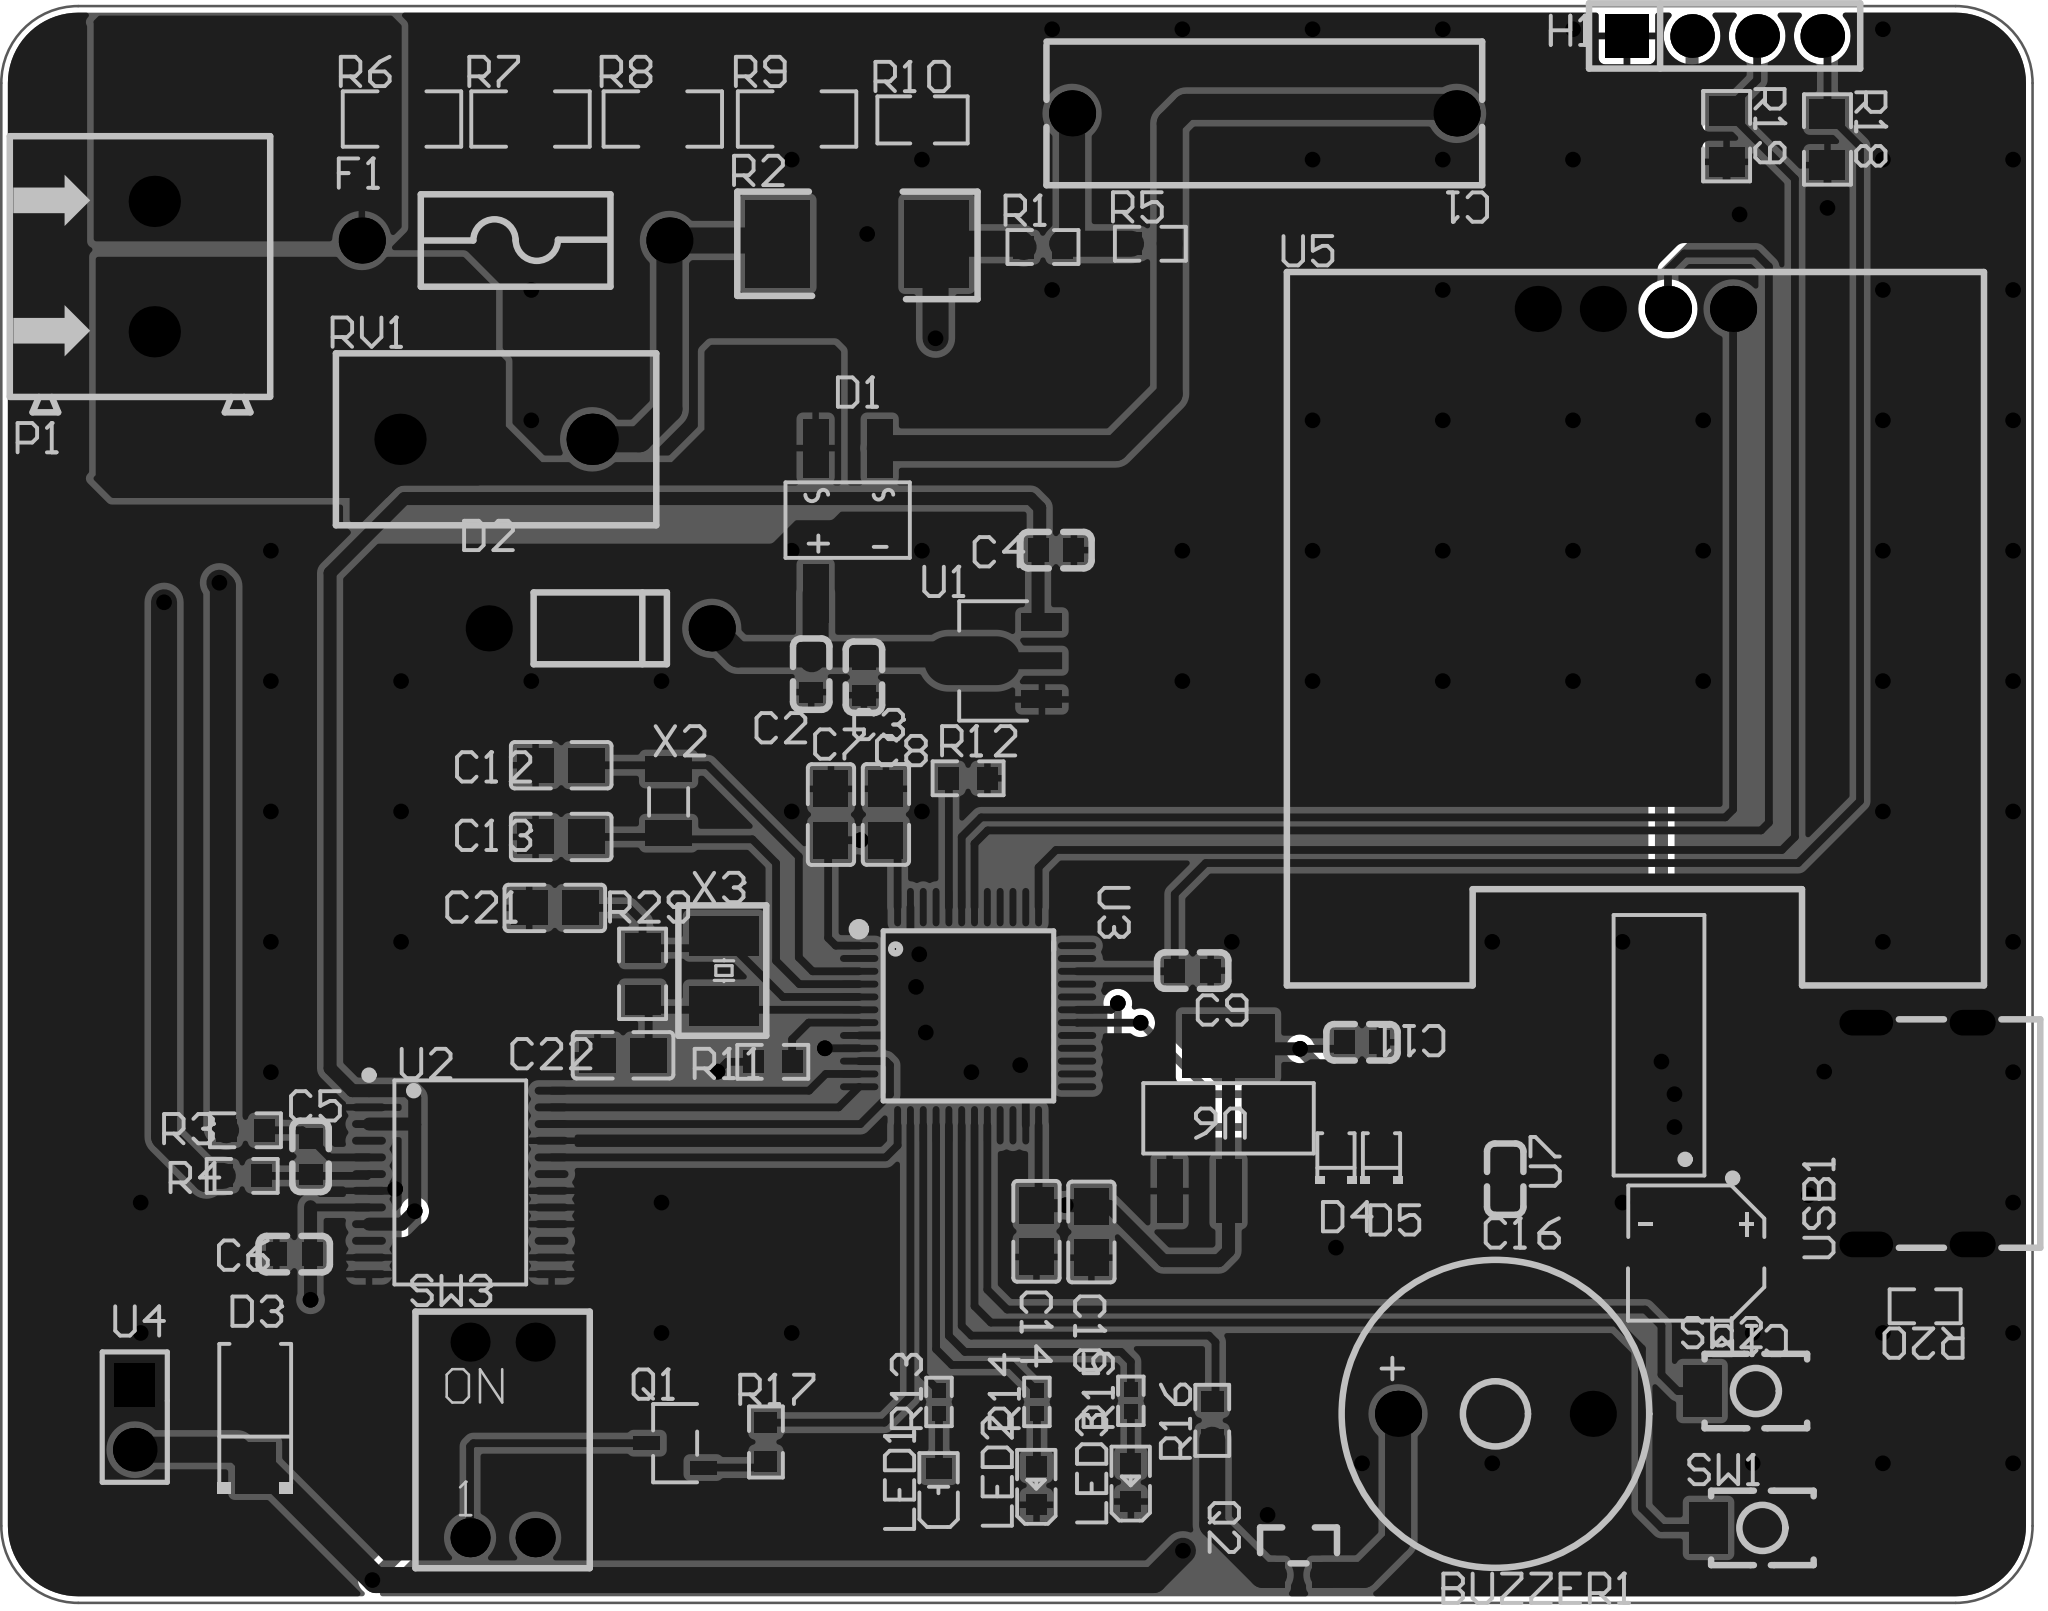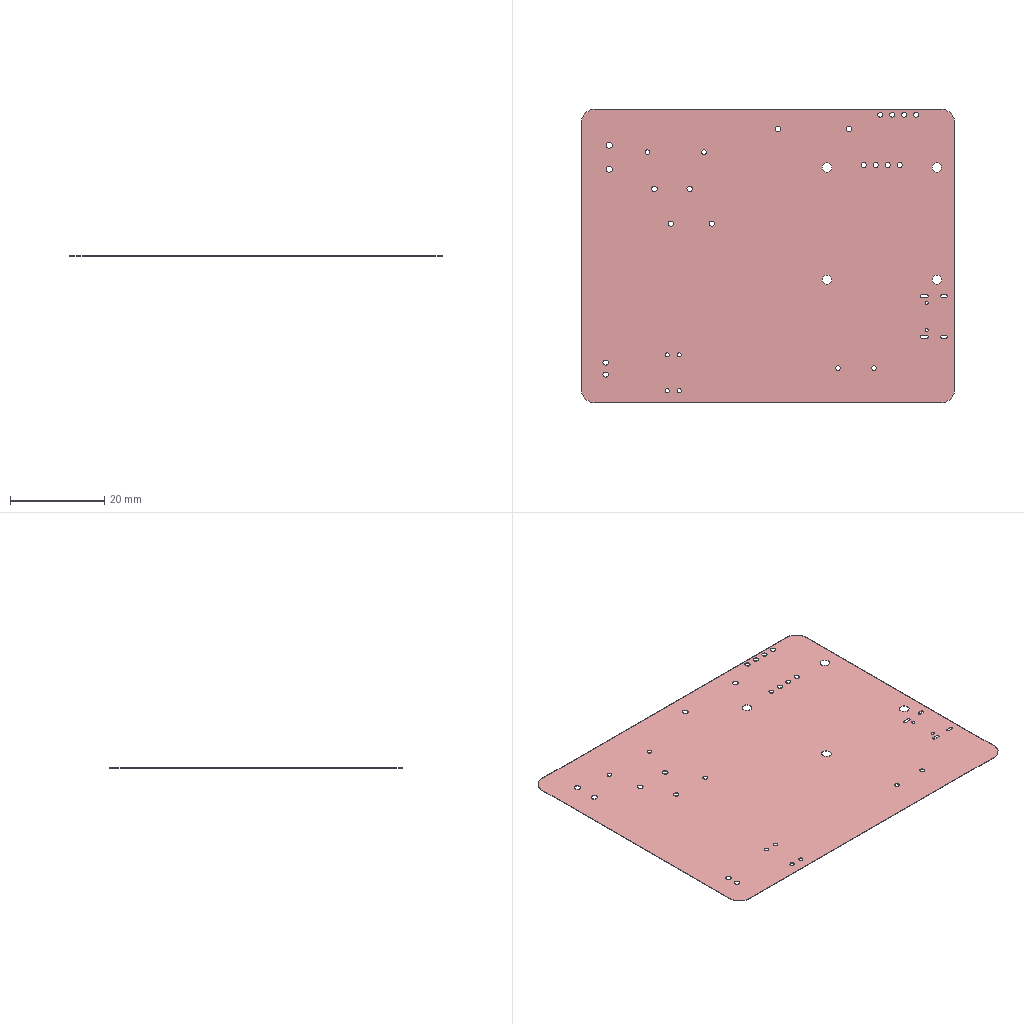Circuit board layout | Altium Designer | box 79.2 x 62.2 x 0.1 mm
Layer stack:
# Altium Designer layer stack of  (unit mm; dielectric type: 0 none, 1 core, 2 prepreg, 3 surface material)
index,name,kind,layer,copper_thickness_mm,dielectric_type,dielectric_thickness_mm,dielectric_material,dielectric_constant
0,Top Paste Mask Layer,other,,,,,,
1,Top Silkscreen Layer,other,,,,,,
2,Top Solder Mask Layer,dielectric,,,3,0.01,,3.3
3,Top Layer,copper,Top Layer,0.035,,,,
4,Bottom Layer,copper,Bottom Layer,0.035,,,,
5,Bottom Solder Mask Layer,dielectric,,,3,0.01,,3.3
6,Bottom Silkscreen Layer,other,,,,,,
7,Bottom Paste Mask Layer,other,,,,,,
# drill layer pairs: low layer,high layer
drill_pair,Top Layer,Bottom Layer
Part placement:
Designator,Comment,Layer,Footprint,Center-X(mm),Center-Y(mm),Rotation
BUZZER1,2.4kHz,TopLayer,BUZ-TH_BD12.0-P7.60-D0.6-FD,140.589,89.281,0
C1,470nF,TopLayer,CAP-TH_L17.0-W5.5-P15.00-D1.2,131.572,139.954,180
C3,0.1µF,TopLayer,C0603,115.951,117.983,270
C4,10µF,TopLayer,C0603,123.444,122.936,180
C5,1nF,TopLayer,C0603,94.361,99.314,90
C6,1nF,TopLayer,C0603,93.726,95.504,0
C7,100nF,TopLayer,C0805,114.665,112.633,90
C8,100nF,TopLayer,C0805,116.809,112.637,270
C14,100nF,TopLayer,C0805,122.682,96.393,90
C10,100nF,TopLayer,C0805,124.825,96.367,270
C11,100nF,TopLayer,C0603,135.382,103.759,180
D1,MB10S,TopLayer,MBS_L4.7-W4.0-P2.50-LS7.0-TL,115.316,124.079,270
D2,1N4742,TopLayer,DO-41_BD2.4-L4.7-P8.70-D0.8-FD,105.664,119.888,0
D3,1N4007,TopLayer,SMA_L4.3-W2.5-LS5.0-RD,92.202,89.281,90
F1,2F0.05002S1B02,TopLayer,FUSE-TH_BD3.0-L7.2-P11.20-D0.6,102.362,135.001,0
LED1,NCD0603G1,TopLayer,LED0603-RD_1,118.869,86.361,90
LED2,NCD0603R1,TopLayer,LED0603-RD_RED,122.682,86.487,90
LED3,NCD0603Y1,TopLayer,LED0603-RD,126.365,86.614,90
Q1,S8050 J3Y(RANGE:200-350),TopLayer,SOT-23-3_L3.0-W1.7-P0.95-LS2.9-BR,108.585,88.138,0
R1,10Ω,TopLayer,R0603,122.936,134.747,0
R2,2mΩ,TopLayer,RES-SMD_L6.4-W3.2-1,115.697,134.874,0
R3,1K,TopLayer,R0603,91.821,100.33,0
R4,1K,TopLayer,R0603,91.694,98.552,0
R5,1MΩ,TopLayer,R0603,127.127,134.874,0
R6,1MΩ,TopLayer,R1206,97.928,139.734,0
R7,1MΩ,TopLayer,R1206,102.943,139.734,0
R8,1MΩ,TopLayer,R1206,108.104,139.734,0
R9,1MΩ,TopLayer,R1206,113.342,139.734,0
R11,10K,TopLayer,R0603,112.395,102.997,0
R12,10K,TopLayer,R0603,120.015,114.046,0
R13,220Ω,TopLayer,R0402,118.879,89.745,90
R14,220Ω,TopLayer,R0402,122.7,89.745,90
R15,220Ω,TopLayer,R0402,126.365,89.789,90
R16,1KΩ,TopLayer,R0603,129.54,89.027,90
R17,1KΩ,TopLayer,R0603,112.128,88.184,270
RV1,190pF@1kHz,TopLayer,RES-TH_L12.5-W6.7-P7.50-D1.2,101.6,127.254,0
SW1,TS3425A2P 250gf,TopLayer,SW-SMD_L3.9-W2.9-LS5.0,151.003,84.836,0
SW2,TS3425A2P 250gf,TopLayer,SW-SMD_L3.9-W2.9-LS5.0,150.749,90.17,0
SW3,BSE02GR,TopLayer,SW-TH_4P-L9.9-W6.8-P7.62-BL,101.854,88.265,0
U1,HT7550-1,TopLayer,SOT-89_L4.5-W2.5-P1.50-LS4.2-BR,121.734,118.618,0
U2,ADE7755ARSZ,TopLayer,SSOP-24_L8.1-W5.3-P0.65-LS7.8-BL,100.203,98.298,270
U3,STM32F030C8T6TR,TopLayer,LQFP-48_L7.0-W7.0-P0.50-LS9.0-BL,120.015,104.775,270
U5,HS96L03W2C03,TopLayer,OLED-TH_L27.8-W27.2-P2.54_C9900033791,146.05,132.334,0
U6,AMS1117-3.3,TopLayer,SOT-223-4_L6.5-W3.5-P2.30-LS7.0-BR,130.175,100.796,270
P1,WJ500V-5.08-2P,TopLayer,CONN-TH_2P-P5.00_WJ500V-5.08-2P,88.265,133.985,90
U4,KF301-5.0-2P,TopLayer,HDR-M-2.54_1X2,87.503,89.154,270
C12,20pF,TopLayer,C0805,104.14,114.554,180
C13,20pF,TopLayer,C0805,104.14,111.76,0
C21,20pF,TopLayer,C0805,103.891,108.994,0
C22,20pF,TopLayer,C0805,106.553,103.251,0
R29,1M,TopLayer,R0805,107.315,106.426,90
X3,8MHz,TopLayer,CRYSTAL-SMD_L3.2-W2.5_3225-8MHZ,110.49,106.553,90
C9,100nF,TopLayer,C0603,128.778,106.553,180
C16,100nF,TopLayer,C0603,140.97,98.425,90
R18,10kΩ,TopLayer,R0805,153.543,138.938,270
R19,10kΩ,TopLayer,R0805,149.606,139.065,270
R20,5.1K,TopLayer,R0603,157.353,93.472,180
U7,CH340C,TopLayer,SOP-16_L10.0-W3.9-P1.27-LS6.0-BL,146.97,103.642,90
USB1,TYPE-C16PIN,TopLayer,USB-C-SMD_TYPE-C16PIN,156.845,100.203,90
Q2,,TopLayer,S8050_SOT-23,132.906,84.154,270
H1,,TopLayer,HDR-TH_4P-P2.54-V-F,149.53,142.971,0
D4,1N5819WS,TopLayer,SOD-323_L1.8-W1.3-LS2.5-RD,134.366,99.314,90
D5,1N5819WS,TopLayer,SOD-323_L1.8-W1.3-LS2.5-RD,136.144,99.314,90
C2,47uF,TopLayer,C0603,113.894,118.104,270
C15,10uF,TopLayer,CAP-SMD_BD5.0-L5.3-W5.3-FD,148.42,95.561,180
R10,10kΩ,TopLayer,R0805,118.237,139.7,0
X2,32.768kHz,TopLayer,CRYSTAL-SMD_L3.2-W1.5-FC-135R32.768KF-A3,108.331,113.157,270
Pad and via stacks:
# Altium Designer via and pad stacks of  (unit mm). Each distinct definition once, with the count of objects using it.
# via: kind,start_layer,end_layer,hole_mm,diameter_mm,mode(0 simple;1 top-mid-bottom;2 full stack),diameter_per_layer,count,example_net
# pad: kind,layer,hole_mm,hole_type(0 round;1 square;2 slot),plating,top_size,top_shape(1 round;2 rect;3 octagon;9 rounded rect),mid_size,bottom_size,mode,footprint,size_per_layer,count,example
pad,Multi-Layer,1,0,plated,1.8x1.8,1,1.8x1.8,1.8x1.8,0,BUZ-TH_BD12.0-P7.60-D0.6-FD,,2,BUZZER1.2
pad,Multi-Layer,1.2,0,plated,1.8x1.8,1,1.8x1.8,1.8x1.8,0,CAP-TH_L17.0-W5.5-P15.00-D1.2,,2,C1.1
pad,Multi-Layer,1.1,0,plated,1.8x1.8,1,1.8x1.8,1.8x1.8,0,DO-41_BD2.4-L4.7-P8.70-D0.8-FD,,2,D2.1
pad,Multi-Layer,1,0,plated,1.8x1.8,1,1.8x1.8,1.8x1.8,0,FUSE-TH_BD3.0-L7.2-P11.20-D0.6,,2,F1.1
pad,Multi-Layer,1.2,0,plated,2x2,1,2x2,2x2,0,RES-TH_L12.5-W6.7-P7.50-D1.2,,2,RV1.1
pad,Multi-Layer,0.9144,0,plated,1.524x1.524,1,1.524x1.524,1.524x1.524,0,SW-TH_4P-L9.9-W6.8-P7.62-BL,,4,SW3.1
pad,Multi-Layer,1.05,0,plated,1.8x1.8,1,1.8x1.8,1.8x1.8,0,OLED-TH_L27.8-W27.2-P2.54_C9900033791,,4,U5.1
pad,Multi-Layer,1.3,0,plated,2x2,1,2x2,2x2,0,CONN-TH_2P-P5.00_WJ500V-5.08-2P,,2,P1.2
pad,Multi-Layer,1.1,0,plated,1.7x1.575,2,1.7x1.575,1.7x1.575,0,HDR-M-2.54_1X2,,1,U4.1
pad,Multi-Layer,1.1,0,plated,1.7x1.7,1,1.7x1.7,1.7x1.7,0,HDR-M-2.54_1X2,,1,U4.2
pad,Multi-Layer,0.6,2,plated,1x1.8,1,1x1.8,1x1.8,0,USB-C-SMD_TYPE-C16PIN,,2,USB1.4
pad,Multi-Layer,0.6,2,plated,1x2.1,1,1x2.1,1x2.1,0,USB-C-SMD_TYPE-C16PIN,,2,USB1.2
pad,Multi-Layer,1.1,0,plated,1.7x1.7,2,1.7x1.7,1.7x1.7,0,HDR-TH_4P-P2.54-V-F,,1,H1.1
pad,Multi-Layer,1.1,0,plated,1.7x1.7,1,1.7x1.7,1.7x1.7,0,HDR-TH_4P-P2.54-V-F,,3,H1.2
pad,Top Layer,0,0,plated,0.8x0.9,2,0.8x0.9,0.8x0.9,0,C0603,,16,C3.2
pad,Top Layer,0,0,plated,1.41x1.35,2,1.41x1.35,1.41x1.35,0,C0805,,16,C7.2
pad,Top Layer,0,0,plated,0.98x2.265,2,0.98x2.265,0.98x2.265,0,MBS_L4.7-W4.0-P2.50-LS7.0-TL,,4,D1.1
pad,Top Layer,0,0,plated,2x1.593,2,2x1.593,2x1.593,0,SMA_L4.3-W2.5-LS5.0-RD,,2,D3.2
pad,Top Layer,0,0,plated,1x0.8,2,1x0.8,1x0.8,0,LED0603-RD_1,,2,LED1.2
pad,Top Layer,0,0,plated,0.8x0.8,2,0.8x0.8,0.8x0.8,0,LED0603-RD_RED,,2,LED2.1
pad,Top Layer,0,0,plated,0.8x0.8,2,0.8x0.8,0.8x0.8,0,LED0603-RD,,2,LED3.2
pad,Top Layer,0,0,plated,1.038x0.532,2,1.038x0.532,1.038x0.532,0,SOT-23-3_L3.0-W1.7-P0.95-LS2.9-BR,,3,Q1.1
pad,Top Layer,0,0,plated,0.8065x0.864,2,0.8065x0.864,0.8065x0.864,0,R0603,,18,R1.2
pad,Top Layer,0,0,plated,2.5x3.4,2,2.5x3.4,2.5x3.4,0,RES-SMD_L6.4-W3.2-1,,2,R2.2
pad,Top Layer,0,0,plated,1.208x1.701,2,1.208x1.701,1.208x1.701,0,R1206,,8,R6.2
pad,Top Layer,0,0,plated,0.5657x0.54,2,0.5657x0.54,0.5657x0.54,0,R0402,,6,R13.2
pad,Top Layer,0,0,plated,1.5x2,2,1.5x2,1.5x2,0,SW-SMD_L3.9-W2.9-LS5.0,,4,SW1.1
pad,Top Layer,0,0,plated,0.95x0.95,1,0.95x0.95,0.95x0.95,0,SOT-89_L4.5-W2.5-P1.50-LS4.2-BR,,1,U1.2
pad,Top Layer,0,0,plated,1.575x0.672,2,1.575x0.672,1.575x0.672,0,SOT-89_L4.5-W2.5-P1.50-LS4.2-BR,,2,U1.3
pad,Top Layer,0,0,plated,0.308x1.324,1,0.308x1.324,0.308x1.324,0,SSOP-24_L8.1-W5.3-P0.65-LS7.8-BL,,24,U2.1
pad,Top Layer,0,0,plated,0.27x1.5,1,0.27x1.5,0.27x1.5,0,LQFP-48_L7.0-W7.0-P0.50-LS9.0-BL,,24,U3.1
pad,Top Layer,0,0,plated,1.5x0.27,1,1.5x0.27,1.5x0.27,0,LQFP-48_L7.0-W7.0-P0.50-LS9.0-BL,,24,U3.13
pad,Top Layer,0,0,plated,2.47x0.98,2,2.47x0.98,2.47x0.98,0,SOT-223-4_L6.5-W3.5-P2.30-LS7.0-BR,,3,U6.1
pad,Top Layer,0,0,plated,2.47x3.6,2,2.47x3.6,2.47x3.6,0,SOT-223-4_L6.5-W3.5-P2.30-LS7.0-BR,,1,U6.4
pad,Top Layer,0,0,plated,1.133x1.377,2,1.133x1.377,1.133x1.377,0,R0805,,8,R29.2
pad,Top Layer,0,0,plated,1.524x2.7,2,1.524x2.7,1.524x2.7,0,CRYSTAL-SMD_L3.2-W2.5_3225-8MHZ,,2,X3.1
pad,Top Layer,0,0,plated,0.56x1.745,1,0.56x1.745,0.56x1.745,0,SOP-16_L10.0-W3.9-P1.27-LS6.0-BL,,16,U7.1
pad,Top Layer,0,0,plated,0.6x1.15,2,0.6x1.15,0.6x1.15,0,USB-C-SMD_TYPE-C16PIN,,4,USB1.A1B12
pad,Top Layer,0,0,plated,0.3x1.15,2,0.3x1.15,0.3x1.15,0,USB-C-SMD_TYPE-C16PIN,,8,USB1.B5
pad,Top Layer,0,0,plated,1x0.8,2,1x0.8,1x0.8,0,S8050_SOT-23,,3,Q2.2
pad,Top Layer,0,0,plated,1x0.75,2,1x0.75,1x0.75,0,SOD-323_L1.8-W1.3-LS2.5-RD,,4,D4.1
pad,Top Layer,0,0,plated,2.8x1.1,2,2.8x1.1,2.8x1.1,0,CAP-SMD_BD5.0-L5.3-W5.3-FD,,2,C15.1
pad,Top Layer,0,0,plated,1x1.8,2,1x1.8,1x1.8,0,CRYSTAL-SMD_L3.2-W1.5-FC-135R32.768KF-A3,,2,X2.2
via,Top Layer,Bottom Layer,0.3048,0.6096,0,,106,TT1
Copper pours:
name,layer,net,type(0 solid;1 hatched;2 none)
Top Layer-$1N1,Top Layer,$1N1,0
Top Layer-$1N67,Top Layer,$1N67,0
Top Layer-$1N68,Top Layer,$1N68,0
Top Layer-$1N69,Top Layer,$1N69,0
Top Layer-VDDS,Top Layer,VDDS,0
Top Layer-$1N109,Top Layer,$1N109,0
Top Layer-$1N109 1,Top Layer,$1N109,0
Top Layer-GND,Top Layer,GND,0
Bottom Layer-GND,Bottom Layer,GND,0
Design rules, without the lines most boards share:
# Altium Designer design rules of  (exported by Altium Designer, unit mm)
# columns: name | kind | enabled | priority | scope1 | scope2 | descriptor | typed fields (field=value)
Plane_innerPlane | 0 | disabled | 1 | All | All | Clearance Constraint (Gap=6mil) (Disabled)(All),(All) | gap=0.1524
Plane_innerPlane_1 | 63 | disabled | 1 | All | All | Board Clearance Constraint (Gap=0mil) (Disabled)(All) |
Copper_copperRegion | 0 | disabled | 2 | All | All | Clearance Constraint (Gap=6mil) (Disabled)(All),(All) | gap=0.1524
Copper_copperRegion_1 | 63 | disabled | 2 | All | All | Board Clearance Constraint (Gap=0mil) (Disabled)(All) |
Copper_copperRegion_copperThickness1oz | 0 | disabled | 3 | All | All | Clearance Constraint (Gap=6mil) (Disabled)(All),(All) | gap=0.1524
Copper_copperRegion_copperThickness1oz_1 | 63 | disabled | 3 | All | All | Board Clearance Constraint (Gap=0mil) (Disabled)(All) |
Copper_copperRegion_Copper_copperRegion | 0 | disabled | 4 | All | All | Clearance Constraint (Gap=6mil) (Disabled)(All),(All) | gap=0.1524
Copper_copperRegion_Copper_copperRegion_1 | 63 | disabled | 4 | All | All | Board Clearance Constraint (Gap=0mil) (Disabled)(All) |
copperThickness1oz | 0 | enabled | 5 | All | All | Clearance Constraint (Gap=6mil) (All),(All) | gap=0.1524
copperThickness1oz_1 | 63 | enabled | 5 | All | All | Board Clearance Constraint (Gap=0mil) (All) |
otherClearance | 52 | enabled | 1 | All | All | Hole To Hole Clearance (Gap=11.8mil) (All),(All) | gap=0.2997
copperThickness1oz_2 | 2 | enabled | 1 | All | All | Width Constraint (Min=5mil) (Max=100mil) (Preferred=10mil) (All) |
differentialPair | 51 | enabled | 1 | All | All | Differential Pairs Uncoupled Length using the Gap Constraints (Min=5mil) (Max=6mil) (Prefered=6mil)  and Width Constraints (Min=5mil) (Max=100mil) (Prefered=100mil) (All) |
viaSize | 11 | enabled | 1 | All | All | Routing Via (MinHoleWidth=1mil) (MaxHoleWidth=393.7mil) (PreferredHoleWidth=12mil) (MinWidth=1mil) (MaxWidth=248mil) (PreferedWidth=24mil) (All) | via_min_hole=0.0254 via_max_hole=10 via_preferred_diameter=0.6096 via_preferred_hole=0.3048
copperRegion_copperThickness1oz | 20 | disabled | 1 | All | All | Polygon Connect Rule(Relief Connect )(Conductor Width=10mil) (Relief Angle=90 Angle) (Entries=4) (Air Gap Width=10mil) (Disabled)(All),(All) | connect_style(0=relief,1=direct,2=none)=0 relief_conductor_width=0.254 relief_entries=4
copperRegion_Copper_copperRegion | 20 | disabled | 2 | All | All | Polygon Connect Rule(Relief Connect )(Conductor Width=10mil) (Relief Angle=90 Angle) (Entries=4) (Air Gap Width=10mil) (Disabled)(All),(All) | connect_style(0=relief,1=direct,2=none)=0 relief_conductor_width=0.254 relief_entries=4
copperRegion | 20 | enabled | 3 | All | All | Polygon Connect Rule(Direct Connect )(Conductor Width=10mil) (Relief Angle=90 Angle) (Entries=4) (Air Gap Width=10mil) (All),(All) | connect_style(0=relief,1=direct,2=none)=1 relief_conductor_width=0.254 relief_entries=4